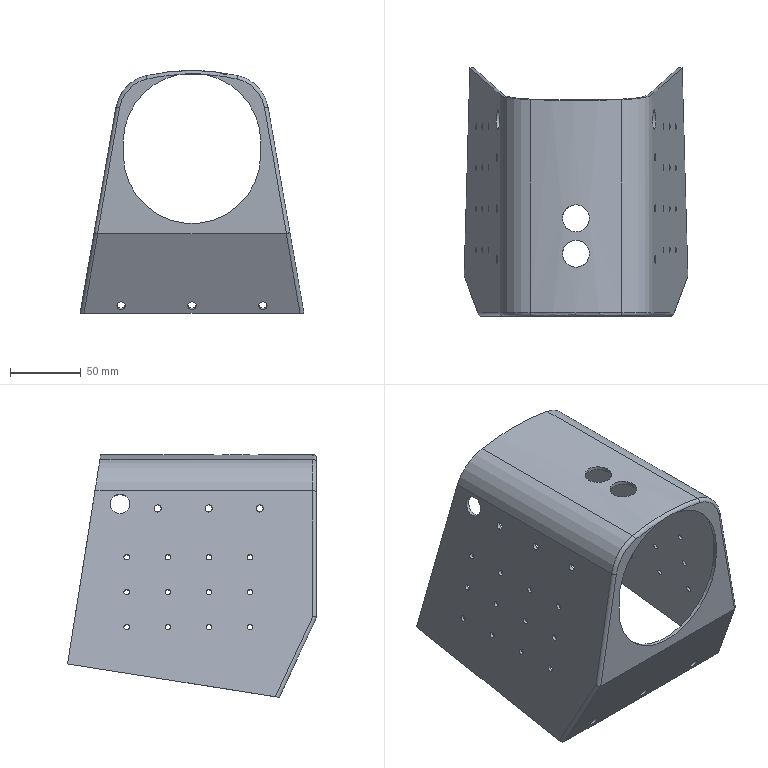Part | STEP file | 1-56.8 | 1 solid | 65 faces | box 157.85 x 175.6 x 171.3 mm | volume 188162 mm3 | cylinder 49 | plane 13 | torus 3 | commonest cylinder face diameters 4 x24 5 x10 6 x3 14 x2 19 x2 50 x2